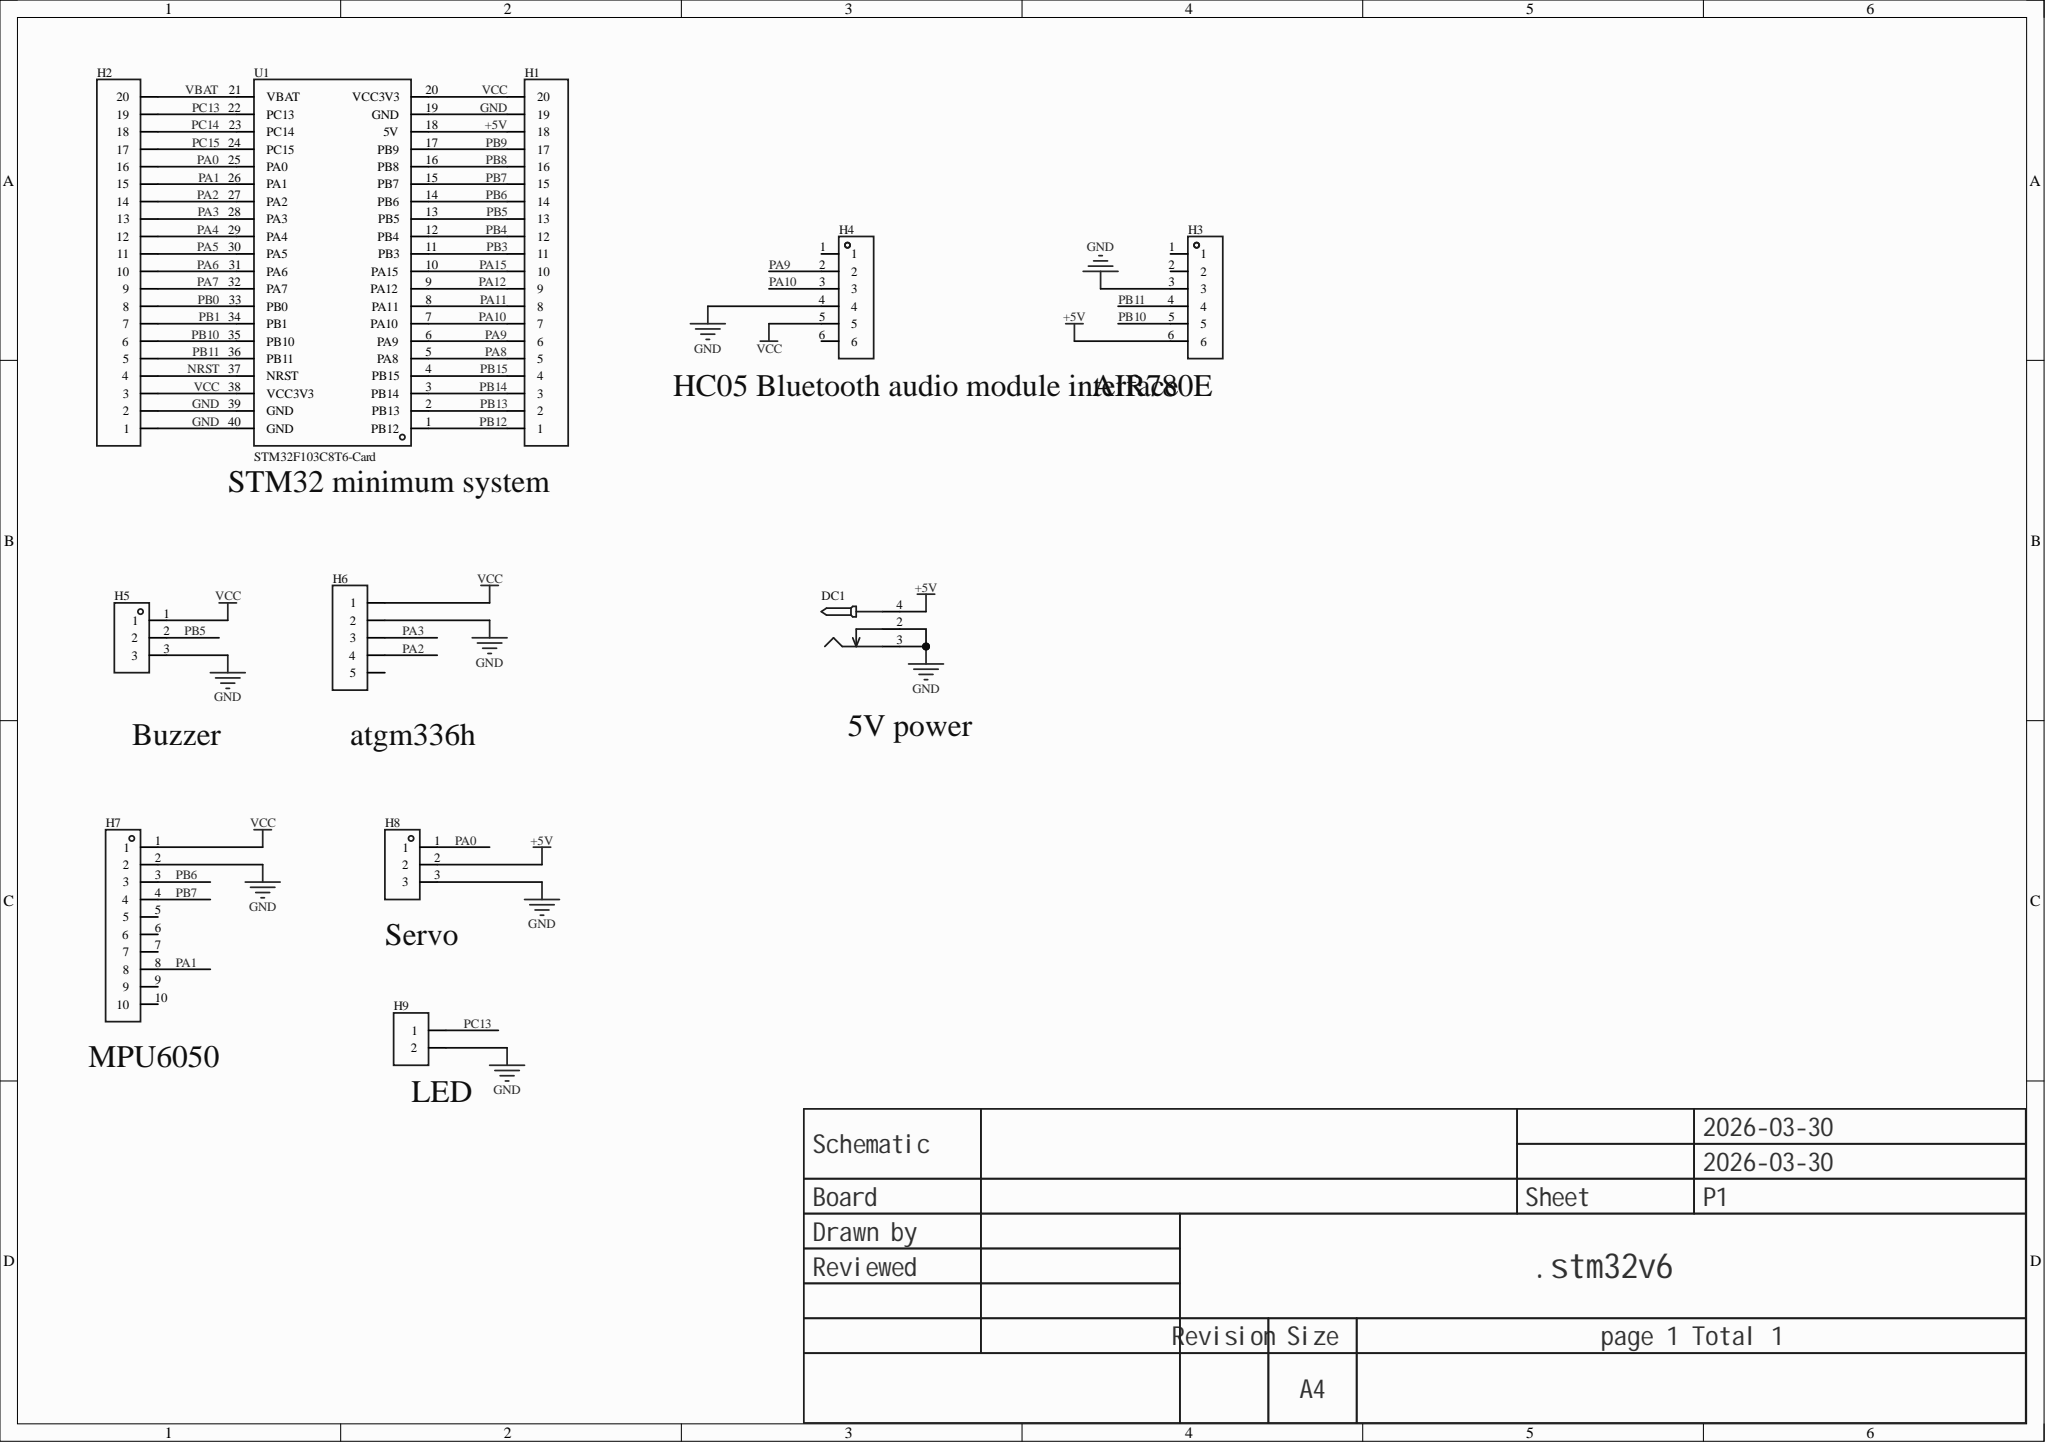Circuit board | Altium Designer | 11 parts | 37 nets
Bill of materials:
Comment,Description,Designator,Footprint,LibRef,Quantity
"","","DC1","DC-2.0","DC-005_2.0","1"
"","","H1, H2","HDR-TH_20P-P2.54-V-F","HDR-F_2.54_1x20P","2"
"","","H3, H4","HDR-TH_6P-P2.54-V-F","HDR-F_2.54_1x6P","2"
"","","H5","HDR-TH_3P-P2.54-V-F","HDR-F_2.54_1x3P","1"
"","","H6","HDR-TH_5P-P2.54-V-F","HDR-F_2.54_1x5P","1"
"","","H7","HDR-TH_10P-P2.54-V-F","HDR-F_2.54_1x10P","1"
"","","H8","HDR-TH_3P-P2.54-V-M","HDR-M_2.54_1x3P","1"
"","","H9","HDR-TH_2P-P2.54-V-F","HDR-F_2.54_1x2P","1"
"STM32F103C8T6-Card","","U1","CONN-TH_L53.3-W22.9_STM32F103C8T6-CARD","STM32F103C8T6-Card","1"
Netlist (Protel format):
[
DC1
DC-2.0




]
[
H1
HDR-TH_20P-P2.54-V-F




]
[
H2
HDR-TH_20P-P2.54-V-F




]
[
H3
HDR-TH_6P-P2.54-V-F




]
[
H4
HDR-TH_6P-P2.54-V-F




]
[
H5
HDR-TH_3P-P2.54-V-F




]
[
H6
HDR-TH_5P-P2.54-V-F




]
[
H7
HDR-TH_10P-P2.54-V-F




]
[
H8
HDR-TH_3P-P2.54-V-M




]
[
H9
HDR-TH_2P-P2.54-V-F




]
[
U1
CONN-TH_L53.3-W22.9_STM32F103C8T6-CARD
STM32F103C8T6-Card



]
(
VCC
H1-20
H2-3
H4-5
H5-1
H6-1
H7-1
U1-20
U1-38
)
(
VBAT
H2-20
U1-21
)
(
PC15
H2-17
U1-24
)
(
PC14
H2-18
U1-23
)
(
PC13
H2-19
H9-1
U1-22
)
(
PB15
H1-4
U1-4
)
(
PB14
H1-3
U1-3
)
(
PB13
H1-2
U1-2
)
(
PB12
H1-1
U1-1
)
(
PB11
H2-5
H3-4
U1-36
)
(
PB10
H2-6
H3-5
U1-35
)
(
PB9
H1-17
U1-17
)
(
PB8
H1-16
U1-16
)
(
PB7
H1-15
H7-4
U1-15
)
(
PB6
H1-14
H7-3
U1-14
)
(
PB5
H1-13
H5-2
U1-13
)
(
PB4
H1-12
U1-12
)
(
PB3
H1-11
U1-11
)
(
PB1
H2-7
U1-34
)
(
PB0
H2-8
U1-33
)
(
PA15
H1-10
U1-10
)
(
PA12
H1-9
U1-9
)
(
PA11
H1-8
U1-8
)
(
PA10
H1-7
H4-3
U1-7
)
(
PA9
H1-6
H4-2
U1-6
)
(
PA8
H1-5
U1-5
)
(
PA7
H2-9
U1-32
)
(
PA6
H2-10
U1-31
)
(
PA5
H2-11
U1-30
)
(
PA4
H2-12
U1-29
)
(
PA3
H2-13
H6-3
U1-28
)
(
PA2
H2-14
H6-4
U1-27
)
(
PA1
H2-15
H7-8
U1-26
)
(
PA0
H2-16
H8-1
U1-25
)
(
NRST
H2-4
U1-37
)
(
GND
DC1-2
DC1-3
H1-19
H2-1
H2-2
H3-3
H4-4
H5-3
H6-2
H7-2
H8-3
H9-2
U1-19
U1-39
U1-40
)
(
+5V
DC1-4
H1-18
H3-6
H8-2
U1-18
)